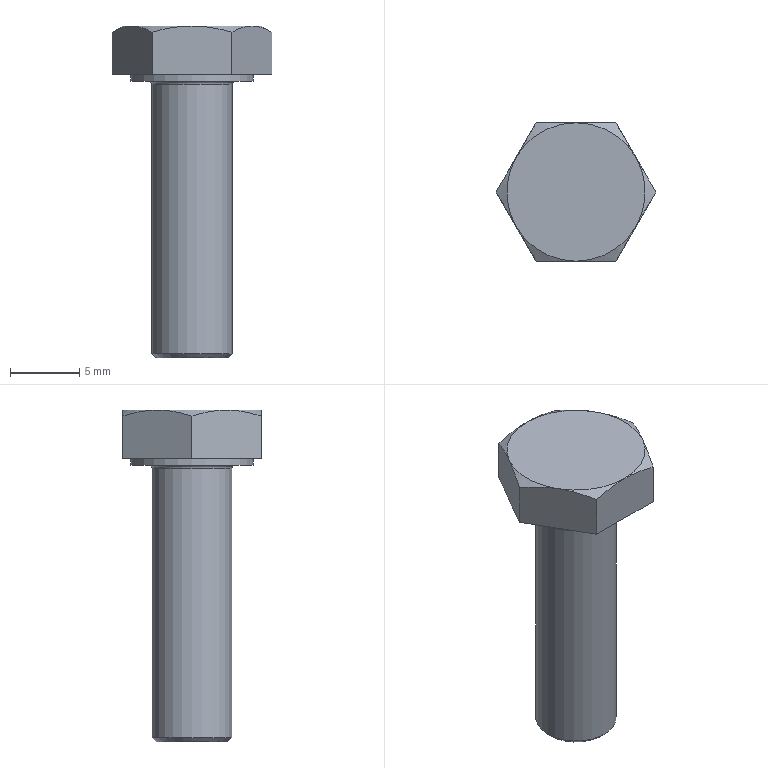Part | NX | 1 solid | 20 faces | box 11.547 x 10 x 24 mm | volume 859.994 mm3 | plane 10 | cone 7 | cylinder 2 | torus 1 | commonest cylinder face diameters 5.795 x1 8.88 x1
STEP:
#1=CARTESIAN_POINT('',(2.887,-5.,3.553));
#2=VERTEX_POINT('',#1);
#3=CARTESIAN_POINT('',(4.33,-2.5,4.));
#4=VERTEX_POINT('',#3);
#5=CARTESIAN_POINT('',(2.887,-5.,3.553));
#6=CARTESIAN_POINT('',(3.358,-4.183,3.826));
#7=CARTESIAN_POINT('',(3.837,-3.353,4.));
#8=CARTESIAN_POINT('',(4.33,-2.5,4.));
#9=B_SPLINE_CURVE_WITH_KNOTS('',3,(#5,#6,#7,#8),.UNSPECIFIED.,.F.,.F.,(4,4),(0.,1.),.UNSPECIFIED.);
#10=EDGE_CURVE('',#2,#4,#9,.T.);
#11=ORIENTED_EDGE('',*,*,#10,.F.);
#12=CARTESIAN_POINT('',(2.887,-5.,0.5));
#13=VERTEX_POINT('',#12);
#14=CARTESIAN_POINT('',(2.887,-5.,4.));
#15=DIRECTION('',(0.,0.,-1.));
#16=VECTOR('',#15,1.);
#17=LINE('',#14,#16);
#18=EDGE_CURVE('',#2,#13,#17,.T.);
#19=ORIENTED_EDGE('',*,*,#18,.T.);
#20=CARTESIAN_POINT('',(5.774,0.,0.5));
#21=VERTEX_POINT('',#20);
#22=CARTESIAN_POINT('',(2.887,-5.,0.5));
#23=DIRECTION('',(0.5,0.866,0.));
#24=VECTOR('',#23,1.);
#25=LINE('',#22,#24);
#26=EDGE_CURVE('',#13,#21,#25,.T.);
#27=ORIENTED_EDGE('',*,*,#26,.T.);
#28=CARTESIAN_POINT('',(5.774,0.,3.553));
#29=VERTEX_POINT('',#28);
#30=CARTESIAN_POINT('',(5.774,0.,4.));
#31=DIRECTION('',(0.,0.,-1.));
#32=VECTOR('',#31,1.);
#33=LINE('',#30,#32);
#34=EDGE_CURVE('',#29,#21,#33,.T.);
#35=ORIENTED_EDGE('',*,*,#34,.F.);
#36=CARTESIAN_POINT('',(4.33,-2.5,4.));
#37=CARTESIAN_POINT('',(4.823,-1.647,4.));
#38=CARTESIAN_POINT('',(5.302,-0.8168,3.826));
#39=CARTESIAN_POINT('',(5.774,0.,3.553));
#40=B_SPLINE_CURVE_WITH_KNOTS('',3,(#36,#37,#38,#39),.UNSPECIFIED.,.F.,.F.,(4,4),(0.,1.),.UNSPECIFIED.);
#41=EDGE_CURVE('',#4,#29,#40,.T.);
#42=ORIENTED_EDGE('',*,*,#41,.F.);
#43=EDGE_LOOP('',(#11,#19,#27,#35,#42));
#44=FACE_OUTER_BOUND('',#43,.T.);
#45=CARTESIAN_POINT('',(2.887,-5.,4.));
#46=DIRECTION('',(-0.866,0.5,0.));
#47=DIRECTION('',(0.5,0.866,0.));
#48=AXIS2_PLACEMENT_3D('',#45,#46,#47);
#49=PLANE('',#48);
#50=ADVANCED_FACE('',(#44),#49,.F.);
#51=CARTESIAN_POINT('',(4.33,2.5,4.));
#52=VERTEX_POINT('',#51);
#53=CARTESIAN_POINT('',(5.774,0.,3.553));
#54=CARTESIAN_POINT('',(5.302,0.8168,3.826));
#55=CARTESIAN_POINT('',(4.823,1.647,4.));
#56=CARTESIAN_POINT('',(4.33,2.5,4.));
#57=B_SPLINE_CURVE_WITH_KNOTS('',3,(#53,#54,#55,#56),.UNSPECIFIED.,.F.,.F.,(4,4),(0.,1.),.UNSPECIFIED.);
#58=EDGE_CURVE('',#29,#52,#57,.T.);
#59=ORIENTED_EDGE('',*,*,#58,.F.);
#60=ORIENTED_EDGE('',*,*,#34,.T.);
#61=CARTESIAN_POINT('',(2.887,5.,0.5));
#62=VERTEX_POINT('',#61);
#63=CARTESIAN_POINT('',(5.774,0.,0.5));
#64=DIRECTION('',(-0.5,0.866,0.));
#65=VECTOR('',#64,1.);
#66=LINE('',#63,#65);
#67=EDGE_CURVE('',#21,#62,#66,.T.);
#68=ORIENTED_EDGE('',*,*,#67,.T.);
#69=CARTESIAN_POINT('',(2.887,5.,3.553));
#70=VERTEX_POINT('',#69);
#71=CARTESIAN_POINT('',(2.887,5.,4.));
#72=DIRECTION('',(0.,0.,-1.));
#73=VECTOR('',#72,1.);
#74=LINE('',#71,#73);
#75=EDGE_CURVE('',#70,#62,#74,.T.);
#76=ORIENTED_EDGE('',*,*,#75,.F.);
#77=CARTESIAN_POINT('',(4.33,2.5,4.));
#78=CARTESIAN_POINT('',(3.837,3.353,4.));
#79=CARTESIAN_POINT('',(3.358,4.183,3.826));
#80=CARTESIAN_POINT('',(2.887,5.,3.553));
#81=B_SPLINE_CURVE_WITH_KNOTS('',3,(#77,#78,#79,#80),.UNSPECIFIED.,.F.,.F.,(4,4),(0.,1.),.UNSPECIFIED.);
#82=EDGE_CURVE('',#52,#70,#81,.T.);
#83=ORIENTED_EDGE('',*,*,#82,.F.);
#84=EDGE_LOOP('',(#59,#60,#68,#76,#83));
#85=FACE_OUTER_BOUND('',#84,.T.);
#86=CARTESIAN_POINT('',(5.774,0.,4.));
#87=DIRECTION('',(-0.866,-0.5,0.));
#88=DIRECTION('',(-0.5,0.866,0.));
#89=AXIS2_PLACEMENT_3D('',#86,#87,#88);
#90=PLANE('',#89);
#91=ADVANCED_FACE('',(#85),#90,.F.);
#92=CARTESIAN_POINT('',(0.,5.,4.));
#93=VERTEX_POINT('',#92);
#94=CARTESIAN_POINT('',(2.887,5.,3.553));
#95=CARTESIAN_POINT('',(1.944,5.,3.826));
#96=CARTESIAN_POINT('',(0.9853,5.,4.));
#97=CARTESIAN_POINT('',(0.,5.,4.));
#98=B_SPLINE_CURVE_WITH_KNOTS('',3,(#94,#95,#96,#97),.UNSPECIFIED.,.F.,.F.,(4,4),(0.,1.),.UNSPECIFIED.);
#99=EDGE_CURVE('',#70,#93,#98,.T.);
#100=ORIENTED_EDGE('',*,*,#99,.F.);
#101=ORIENTED_EDGE('',*,*,#75,.T.);
#102=CARTESIAN_POINT('',(-2.887,5.,0.5));
#103=VERTEX_POINT('',#102);
#104=CARTESIAN_POINT('',(2.887,5.,0.5));
#105=DIRECTION('',(-1.,0.,0.));
#106=VECTOR('',#105,1.);
#107=LINE('',#104,#106);
#108=EDGE_CURVE('',#62,#103,#107,.T.);
#109=ORIENTED_EDGE('',*,*,#108,.T.);
#110=CARTESIAN_POINT('',(-2.887,5.,3.553));
#111=VERTEX_POINT('',#110);
#112=CARTESIAN_POINT('',(-2.887,5.,4.));
#113=DIRECTION('',(0.,0.,-1.));
#114=VECTOR('',#113,1.);
#115=LINE('',#112,#114);
#116=EDGE_CURVE('',#111,#103,#115,.T.);
#117=ORIENTED_EDGE('',*,*,#116,.F.);
#118=CARTESIAN_POINT('',(0.,5.,4.));
#119=CARTESIAN_POINT('',(-0.9853,5.,4.));
#120=CARTESIAN_POINT('',(-1.944,5.,3.826));
#121=CARTESIAN_POINT('',(-2.887,5.,3.553));
#122=B_SPLINE_CURVE_WITH_KNOTS('',3,(#118,#119,#120,#121),.UNSPECIFIED.,.F.,.F.,(4,4),(0.,1.),.UNSPECIFIED.);
#123=EDGE_CURVE('',#93,#111,#122,.T.);
#124=ORIENTED_EDGE('',*,*,#123,.F.);
#125=EDGE_LOOP('',(#100,#101,#109,#117,#124));
#126=FACE_OUTER_BOUND('',#125,.T.);
#127=CARTESIAN_POINT('',(2.887,5.,4.));
#128=DIRECTION('',(0.,-1.,0.));
#129=DIRECTION('',(0.,0.,1.));
#130=AXIS2_PLACEMENT_3D('',#127,#128,#129);
#131=PLANE('',#130);
#132=ADVANCED_FACE('',(#126),#131,.F.);
#133=CARTESIAN_POINT('',(-4.33,2.5,4.));
#134=VERTEX_POINT('',#133);
#135=CARTESIAN_POINT('',(-2.887,5.,3.553));
#136=CARTESIAN_POINT('',(-3.358,4.183,3.826));
#137=CARTESIAN_POINT('',(-3.837,3.353,4.));
#138=CARTESIAN_POINT('',(-4.33,2.5,4.));
#139=B_SPLINE_CURVE_WITH_KNOTS('',3,(#135,#136,#137,#138),.UNSPECIFIED.,.F.,.F.,(4,4),(0.,1.),.UNSPECIFIED.);
#140=EDGE_CURVE('',#111,#134,#139,.T.);
#141=ORIENTED_EDGE('',*,*,#140,.F.);
#142=ORIENTED_EDGE('',*,*,#116,.T.);
#143=CARTESIAN_POINT('',(-5.774,0.,0.5));
#144=VERTEX_POINT('',#143);
#145=CARTESIAN_POINT('',(-2.887,5.,0.5));
#146=DIRECTION('',(-0.5,-0.866,0.));
#147=VECTOR('',#146,1.);
#148=LINE('',#145,#147);
#149=EDGE_CURVE('',#103,#144,#148,.T.);
#150=ORIENTED_EDGE('',*,*,#149,.T.);
#151=CARTESIAN_POINT('',(-5.774,0.,3.553));
#152=VERTEX_POINT('',#151);
#153=CARTESIAN_POINT('',(-5.774,0.,4.));
#154=DIRECTION('',(0.,0.,-1.));
#155=VECTOR('',#154,1.);
#156=LINE('',#153,#155);
#157=EDGE_CURVE('',#152,#144,#156,.T.);
#158=ORIENTED_EDGE('',*,*,#157,.F.);
#159=CARTESIAN_POINT('',(-4.33,2.5,4.));
#160=CARTESIAN_POINT('',(-4.823,1.647,4.));
#161=CARTESIAN_POINT('',(-5.302,0.8168,3.826));
#162=CARTESIAN_POINT('',(-5.774,0.,3.553));
#163=B_SPLINE_CURVE_WITH_KNOTS('',3,(#159,#160,#161,#162),.UNSPECIFIED.,.F.,.F.,(4,4),(0.,1.),.UNSPECIFIED.);
#164=EDGE_CURVE('',#134,#152,#163,.T.);
#165=ORIENTED_EDGE('',*,*,#164,.F.);
#166=EDGE_LOOP('',(#141,#142,#150,#158,#165));
#167=FACE_OUTER_BOUND('',#166,.T.);
#168=CARTESIAN_POINT('',(-2.887,5.,4.));
#169=DIRECTION('',(0.866,-0.5,0.));
#170=DIRECTION('',(-0.5,-0.866,0.));
#171=AXIS2_PLACEMENT_3D('',#168,#169,#170);
#172=PLANE('',#171);
#173=ADVANCED_FACE('',(#167),#172,.F.);
#174=CARTESIAN_POINT('',(-4.33,-2.5,4.));
#175=VERTEX_POINT('',#174);
#176=CARTESIAN_POINT('',(-5.774,0.,3.553));
#177=CARTESIAN_POINT('',(-5.302,-0.8168,3.826));
#178=CARTESIAN_POINT('',(-4.823,-1.647,4.));
#179=CARTESIAN_POINT('',(-4.33,-2.5,4.));
#180=B_SPLINE_CURVE_WITH_KNOTS('',3,(#176,#177,#178,#179),.UNSPECIFIED.,.F.,.F.,(4,4),(0.,1.),.UNSPECIFIED.);
#181=EDGE_CURVE('',#152,#175,#180,.T.);
#182=ORIENTED_EDGE('',*,*,#181,.F.);
#183=ORIENTED_EDGE('',*,*,#157,.T.);
#184=CARTESIAN_POINT('',(-2.887,-5.,0.5));
#185=VERTEX_POINT('',#184);
#186=CARTESIAN_POINT('',(-5.774,0.,0.5));
#187=DIRECTION('',(0.5,-0.866,0.));
#188=VECTOR('',#187,1.);
#189=LINE('',#186,#188);
#190=EDGE_CURVE('',#144,#185,#189,.T.);
#191=ORIENTED_EDGE('',*,*,#190,.T.);
#192=CARTESIAN_POINT('',(-2.887,-5.,3.553));
#193=VERTEX_POINT('',#192);
#194=CARTESIAN_POINT('',(-2.887,-5.,4.));
#195=DIRECTION('',(0.,0.,-1.));
#196=VECTOR('',#195,1.);
#197=LINE('',#194,#196);
#198=EDGE_CURVE('',#193,#185,#197,.T.);
#199=ORIENTED_EDGE('',*,*,#198,.F.);
#200=CARTESIAN_POINT('',(-4.33,-2.5,4.));
#201=CARTESIAN_POINT('',(-3.837,-3.353,4.));
#202=CARTESIAN_POINT('',(-3.358,-4.183,3.826));
#203=CARTESIAN_POINT('',(-2.887,-5.,3.553));
#204=B_SPLINE_CURVE_WITH_KNOTS('',3,(#200,#201,#202,#203),.UNSPECIFIED.,.F.,.F.,(4,4),(0.,1.),.UNSPECIFIED.);
#205=EDGE_CURVE('',#175,#193,#204,.T.);
#206=ORIENTED_EDGE('',*,*,#205,.F.);
#207=EDGE_LOOP('',(#182,#183,#191,#199,#206));
#208=FACE_OUTER_BOUND('',#207,.T.);
#209=CARTESIAN_POINT('',(-5.774,0.,4.));
#210=DIRECTION('',(0.866,0.5,0.));
#211=DIRECTION('',(0.5,-0.866,0.));
#212=AXIS2_PLACEMENT_3D('',#209,#210,#211);
#213=PLANE('',#212);
#214=ADVANCED_FACE('',(#208),#213,.F.);
#215=CARTESIAN_POINT('',(0.,-5.,4.));
#216=VERTEX_POINT('',#215);
#217=CARTESIAN_POINT('',(-2.887,-5.,3.553));
#218=CARTESIAN_POINT('',(-1.944,-5.,3.826));
#219=CARTESIAN_POINT('',(-0.9853,-5.,4.));
#220=CARTESIAN_POINT('',(0.,-5.,4.));
#221=B_SPLINE_CURVE_WITH_KNOTS('',3,(#217,#218,#219,#220),.UNSPECIFIED.,.F.,.F.,(4,4),(0.,1.),.UNSPECIFIED.);
#222=EDGE_CURVE('',#193,#216,#221,.T.);
#223=ORIENTED_EDGE('',*,*,#222,.F.);
#224=ORIENTED_EDGE('',*,*,#198,.T.);
#225=CARTESIAN_POINT('',(-2.887,-5.,0.5));
#226=DIRECTION('',(1.,0.,0.));
#227=VECTOR('',#226,1.);
#228=LINE('',#225,#227);
#229=EDGE_CURVE('',#185,#13,#228,.T.);
#230=ORIENTED_EDGE('',*,*,#229,.T.);
#231=ORIENTED_EDGE('',*,*,#18,.F.);
#232=CARTESIAN_POINT('',(0.,-5.,4.));
#233=CARTESIAN_POINT('',(0.9853,-5.,4.));
#234=CARTESIAN_POINT('',(1.944,-5.,3.826));
#235=CARTESIAN_POINT('',(2.887,-5.,3.553));
#236=B_SPLINE_CURVE_WITH_KNOTS('',3,(#232,#233,#234,#235),.UNSPECIFIED.,.F.,.F.,(4,4),(0.,1.),.UNSPECIFIED.);
#237=EDGE_CURVE('',#216,#2,#236,.T.);
#238=ORIENTED_EDGE('',*,*,#237,.F.);
#239=EDGE_LOOP('',(#223,#224,#230,#231,#238));
#240=FACE_OUTER_BOUND('',#239,.T.);
#241=CARTESIAN_POINT('',(-2.887,-5.,4.));
#242=DIRECTION('',(0.,1.,0.));
#243=DIRECTION('',(1.,0.,0.));
#244=AXIS2_PLACEMENT_3D('',#241,#242,#243);
#245=PLANE('',#244);
#246=ADVANCED_FACE('',(#240),#245,.F.);
#247=CARTESIAN_POINT('',(4.44,0.,0.5));
#248=VERTEX_POINT('',#247);
#249=CARTESIAN_POINT('',(0.,0.,0.5));
#250=DIRECTION('',(0.,0.,1.));
#251=DIRECTION('',(1.,0.,0.));
#252=AXIS2_PLACEMENT_3D('',#249,#250,#251);
#253=CIRCLE('',#252,4.44);
#254=EDGE_CURVE('',#248,#248,#253,.T.);
#255=ORIENTED_EDGE('',*,*,#254,.T.);
#256=EDGE_LOOP('',(#255));
#257=FACE_BOUND('',#256,.T.);
#258=ORIENTED_EDGE('',*,*,#26,.F.);
#259=ORIENTED_EDGE('',*,*,#229,.F.);
#260=ORIENTED_EDGE('',*,*,#190,.F.);
#261=ORIENTED_EDGE('',*,*,#149,.F.);
#262=ORIENTED_EDGE('',*,*,#108,.F.);
#263=ORIENTED_EDGE('',*,*,#67,.F.);
#264=EDGE_LOOP('',(#258,#259,#260,#261,#262,#263));
#265=FACE_BOUND('',#264,.T.);
#266=CARTESIAN_POINT('',(8.66,5.,0.5));
#267=DIRECTION('',(0.,0.,1.));
#268=DIRECTION('',(-1.,0.,0.));
#269=AXIS2_PLACEMENT_3D('',#266,#267,#268);
#270=PLANE('',#269);
#271=ADVANCED_FACE('',(#257,#265),#270,.F.);
#272=ORIENTED_EDGE('',*,*,#10,.T.);
#273=CARTESIAN_POINT('',(0.,0.,4.));
#274=DIRECTION('',(0.,0.,-1.));
#275=DIRECTION('',(-1.,0.,0.));
#276=AXIS2_PLACEMENT_3D('',#273,#274,#275);
#277=CIRCLE('',#276,5.);
#278=EDGE_CURVE('',#4,#216,#277,.T.);
#279=ORIENTED_EDGE('',*,*,#278,.T.);
#280=ORIENTED_EDGE('',*,*,#237,.T.);
#281=EDGE_LOOP('',(#272,#279,#280));
#282=FACE_OUTER_BOUND('',#281,.T.);
#283=CARTESIAN_POINT('',(0.,0.,3.553));
#284=DIRECTION('',(0.,0.,-1.));
#285=DIRECTION('',(1.,0.,0.));
#286=AXIS2_PLACEMENT_3D('',#283,#284,#285);
#287=CONICAL_SURFACE('',#286,5.774,60.);
#288=ADVANCED_FACE('',(#282),#287,.T.);
#289=ORIENTED_EDGE('',*,*,#205,.T.);
#290=ORIENTED_EDGE('',*,*,#222,.T.);
#291=CARTESIAN_POINT('',(0.,0.,4.));
#292=DIRECTION('',(0.,0.,-1.));
#293=DIRECTION('',(-1.,0.,0.));
#294=AXIS2_PLACEMENT_3D('',#291,#292,#293);
#295=CIRCLE('',#294,5.);
#296=EDGE_CURVE('',#216,#175,#295,.T.);
#297=ORIENTED_EDGE('',*,*,#296,.T.);
#298=EDGE_LOOP('',(#289,#290,#297));
#299=FACE_OUTER_BOUND('',#298,.T.);
#300=CARTESIAN_POINT('',(0.,0.,3.553));
#301=DIRECTION('',(0.,0.,-1.));
#302=DIRECTION('',(1.,0.,0.));
#303=AXIS2_PLACEMENT_3D('',#300,#301,#302);
#304=CONICAL_SURFACE('',#303,5.774,60.);
#305=ADVANCED_FACE('',(#299),#304,.T.);
#306=ORIENTED_EDGE('',*,*,#164,.T.);
#307=ORIENTED_EDGE('',*,*,#181,.T.);
#308=CARTESIAN_POINT('',(0.,0.,4.));
#309=DIRECTION('',(0.,0.,-1.));
#310=DIRECTION('',(-1.,0.,0.));
#311=AXIS2_PLACEMENT_3D('',#308,#309,#310);
#312=CIRCLE('',#311,5.);
#313=EDGE_CURVE('',#175,#134,#312,.T.);
#314=ORIENTED_EDGE('',*,*,#313,.T.);
#315=EDGE_LOOP('',(#306,#307,#314));
#316=FACE_OUTER_BOUND('',#315,.T.);
#317=CARTESIAN_POINT('',(0.,0.,3.553));
#318=DIRECTION('',(0.,0.,-1.));
#319=DIRECTION('',(1.,0.,0.));
#320=AXIS2_PLACEMENT_3D('',#317,#318,#319);
#321=CONICAL_SURFACE('',#320,5.774,60.);
#322=ADVANCED_FACE('',(#316),#321,.T.);
#323=ORIENTED_EDGE('',*,*,#123,.T.);
#324=ORIENTED_EDGE('',*,*,#140,.T.);
#325=CARTESIAN_POINT('',(0.,0.,4.));
#326=DIRECTION('',(0.,0.,-1.));
#327=DIRECTION('',(-1.,0.,0.));
#328=AXIS2_PLACEMENT_3D('',#325,#326,#327);
#329=CIRCLE('',#328,5.);
#330=EDGE_CURVE('',#134,#93,#329,.T.);
#331=ORIENTED_EDGE('',*,*,#330,.T.);
#332=EDGE_LOOP('',(#323,#324,#331));
#333=FACE_OUTER_BOUND('',#332,.T.);
#334=CARTESIAN_POINT('',(0.,0.,3.553));
#335=DIRECTION('',(0.,0.,-1.));
#336=DIRECTION('',(1.,0.,0.));
#337=AXIS2_PLACEMENT_3D('',#334,#335,#336);
#338=CONICAL_SURFACE('',#337,5.774,60.);
#339=ADVANCED_FACE('',(#333),#338,.T.);
#340=ORIENTED_EDGE('',*,*,#82,.T.);
#341=ORIENTED_EDGE('',*,*,#99,.T.);
#342=CARTESIAN_POINT('',(0.,0.,4.));
#343=DIRECTION('',(0.,0.,-1.));
#344=DIRECTION('',(-1.,0.,0.));
#345=AXIS2_PLACEMENT_3D('',#342,#343,#344);
#346=CIRCLE('',#345,5.);
#347=EDGE_CURVE('',#93,#52,#346,.T.);
#348=ORIENTED_EDGE('',*,*,#347,.T.);
#349=EDGE_LOOP('',(#340,#341,#348));
#350=FACE_OUTER_BOUND('',#349,.T.);
#351=CARTESIAN_POINT('',(0.,0.,3.553));
#352=DIRECTION('',(0.,0.,-1.));
#353=DIRECTION('',(1.,0.,0.));
#354=AXIS2_PLACEMENT_3D('',#351,#352,#353);
#355=CONICAL_SURFACE('',#354,5.774,60.);
#356=ADVANCED_FACE('',(#350),#355,.T.);
#357=ORIENTED_EDGE('',*,*,#41,.T.);
#358=ORIENTED_EDGE('',*,*,#58,.T.);
#359=CARTESIAN_POINT('',(0.,0.,4.));
#360=DIRECTION('',(0.,0.,-1.));
#361=DIRECTION('',(-1.,0.,0.));
#362=AXIS2_PLACEMENT_3D('',#359,#360,#361);
#363=CIRCLE('',#362,5.);
#364=EDGE_CURVE('',#52,#4,#363,.T.);
#365=ORIENTED_EDGE('',*,*,#364,.T.);
#366=EDGE_LOOP('',(#357,#358,#365));
#367=FACE_OUTER_BOUND('',#366,.T.);
#368=CARTESIAN_POINT('',(0.,0.,3.553));
#369=DIRECTION('',(0.,0.,-1.));
#370=DIRECTION('',(1.,0.,0.));
#371=AXIS2_PLACEMENT_3D('',#368,#369,#370);
#372=CONICAL_SURFACE('',#371,5.774,60.);
#373=ADVANCED_FACE('',(#367),#372,.T.);
#374=ORIENTED_EDGE('',*,*,#330,.F.);
#375=ORIENTED_EDGE('',*,*,#313,.F.);
#376=ORIENTED_EDGE('',*,*,#296,.F.);
#377=ORIENTED_EDGE('',*,*,#278,.F.);
#378=ORIENTED_EDGE('',*,*,#364,.F.);
#379=ORIENTED_EDGE('',*,*,#347,.F.);
#380=EDGE_LOOP('',(#374,#375,#376,#377,#378,#379));
#381=FACE_OUTER_BOUND('',#380,.T.);
#382=CARTESIAN_POINT('',(8.66,5.,4.));
#383=DIRECTION('',(0.,0.,1.));
#384=DIRECTION('',(-1.,0.,0.));
#385=AXIS2_PLACEMENT_3D('',#382,#383,#384);
#386=PLANE('',#385);
#387=ADVANCED_FACE('',(#381),#386,.T.);
#388=ORIENTED_EDGE('',*,*,#254,.F.);
#389=EDGE_LOOP('',(#388));
#390=FACE_BOUND('',#389,.T.);
#391=CARTESIAN_POINT('',(4.44,0.,0.));
#392=VERTEX_POINT('',#391);
#393=CARTESIAN_POINT('',(0.,0.,0.));
#394=DIRECTION('',(0.,0.,1.));
#395=DIRECTION('',(1.,0.,0.));
#396=AXIS2_PLACEMENT_3D('',#393,#394,#395);
#397=CIRCLE('',#396,4.44);
#398=EDGE_CURVE('',#392,#392,#397,.T.);
#399=ORIENTED_EDGE('',*,*,#398,.T.);
#400=EDGE_LOOP('',(#399));
#401=FACE_BOUND('',#400,.T.);
#402=CARTESIAN_POINT('',(0.,0.,0.5));
#403=DIRECTION('',(0.,0.,-1.));
#404=DIRECTION('',(1.,0.,0.));
#405=AXIS2_PLACEMENT_3D('',#402,#403,#404);
#406=CYLINDRICAL_SURFACE('',#405,4.44);
#407=ADVANCED_FACE('',(#390,#401),#406,.T.);
#408=CARTESIAN_POINT('',(3.147,0.,0.));
#409=VERTEX_POINT('',#408);
#410=CARTESIAN_POINT('',(0.,0.,0.));
#411=DIRECTION('',(0.,0.,1.));
#412=DIRECTION('',(1.,0.,0.));
#413=AXIS2_PLACEMENT_3D('',#410,#411,#412);
#414=CIRCLE('',#413,3.147);
#415=EDGE_CURVE('',#409,#409,#414,.T.);
#416=ORIENTED_EDGE('',*,*,#415,.T.);
#417=EDGE_LOOP('',(#416));
#418=FACE_BOUND('',#417,.T.);
#419=ORIENTED_EDGE('',*,*,#398,.F.);
#420=EDGE_LOOP('',(#419));
#421=FACE_BOUND('',#420,.T.);
#422=CARTESIAN_POINT('',(0.,0.,0.));
#423=DIRECTION('',(0.,0.,1.));
#424=DIRECTION('',(-1.,0.,0.));
#425=AXIS2_PLACEMENT_3D('',#422,#423,#424);
#426=PLANE('',#425);
#427=ADVANCED_FACE('',(#418,#421),#426,.F.);
#428=CARTESIAN_POINT('',(2.897,0.,-0.25));
#429=VERTEX_POINT('',#428);
#430=CARTESIAN_POINT('',(0.,0.,-0.25));
#431=DIRECTION('',(0.,0.,-1.));
#432=DIRECTION('',(1.,0.,0.));
#433=AXIS2_PLACEMENT_3D('',#430,#431,#432);
#434=CIRCLE('',#433,2.897);
#435=EDGE_CURVE('',#429,#429,#434,.T.);
#436=ORIENTED_EDGE('',*,*,#435,.T.);
#437=EDGE_LOOP('',(#436));
#438=FACE_BOUND('',#437,.T.);
#439=CARTESIAN_POINT('',(2.897,0.,-19.71));
#440=VERTEX_POINT('',#439);
#441=CARTESIAN_POINT('',(0.,0.,-19.71));
#442=DIRECTION('',(0.,0.,1.));
#443=DIRECTION('',(1.,0.,0.));
#444=AXIS2_PLACEMENT_3D('',#441,#442,#443);
#445=CIRCLE('',#444,2.897);
#446=EDGE_CURVE('',#440,#440,#445,.T.);
#447=ORIENTED_EDGE('',*,*,#446,.T.);
#448=EDGE_LOOP('',(#447));
#449=FACE_BOUND('',#448,.T.);
#450=CARTESIAN_POINT('',(0.,0.,-20.));
#451=DIRECTION('',(0.,0.,1.));
#452=DIRECTION('',(-1.,0.,0.));
#453=AXIS2_PLACEMENT_3D('',#450,#451,#452);
#454=CYLINDRICAL_SURFACE('',#453,2.897);
#455=ADVANCED_FACE('',(#438,#449),#454,.T.);
#456=CARTESIAN_POINT('',(2.608,0.,-20.));
#457=VERTEX_POINT('',#456);
#458=CARTESIAN_POINT('',(0.,0.,-20.));
#459=DIRECTION('',(0.,0.,-1.));
#460=DIRECTION('',(1.,0.,0.));
#461=AXIS2_PLACEMENT_3D('',#458,#459,#460);
#462=CIRCLE('',#461,2.608);
#463=EDGE_CURVE('',#457,#457,#462,.T.);
#464=ORIENTED_EDGE('',*,*,#463,.T.);
#465=EDGE_LOOP('',(#464));
#466=FACE_OUTER_BOUND('',#465,.T.);
#467=CARTESIAN_POINT('',(0.,0.,-20.));
#468=DIRECTION('',(0.,0.,1.));
#469=DIRECTION('',(-1.,0.,0.));
#470=AXIS2_PLACEMENT_3D('',#467,#468,#469);
#471=PLANE('',#470);
#472=ADVANCED_FACE('',(#466),#471,.F.);
#473=ORIENTED_EDGE('',*,*,#463,.F.);
#474=EDGE_LOOP('',(#473));
#475=FACE_BOUND('',#474,.T.);
#476=ORIENTED_EDGE('',*,*,#446,.F.);
#477=EDGE_LOOP('',(#476));
#478=FACE_BOUND('',#477,.T.);
#479=CARTESIAN_POINT('',(0.,0.,-19.71));
#480=DIRECTION('',(0.,0.,1.));
#481=DIRECTION('',(-1.,0.,0.));
#482=AXIS2_PLACEMENT_3D('',#479,#480,#481);
#483=CONICAL_SURFACE('',#482,2.897,45.);
#484=ADVANCED_FACE('',(#475,#478),#483,.T.);
#485=ORIENTED_EDGE('',*,*,#435,.F.);
#486=EDGE_LOOP('',(#485));
#487=FACE_BOUND('',#486,.T.);
#488=ORIENTED_EDGE('',*,*,#415,.F.);
#489=EDGE_LOOP('',(#488));
#490=FACE_BOUND('',#489,.T.);
#491=CARTESIAN_POINT('',(0.,0.,-0.25));
#492=DIRECTION('',(0.,0.,1.));
#493=DIRECTION('',(-1.,0.,0.));
#494=AXIS2_PLACEMENT_3D('',#491,#492,#493);
#495=TOROIDAL_SURFACE('',#494,3.147,0.25);
#496=ADVANCED_FACE('',(#487,#490),#495,.F.);
#497=CLOSED_SHELL('',(#50,#91,#132,#173,#214,#246,#271,#288,#305,#322,#339,#356,#373,#387,#407,#427,#455,#472,#484,#496));
#498=MANIFOLD_SOLID_BREP('',#497);
#499=(LENGTH_UNIT()NAMED_UNIT(*)SI_UNIT(.MILLI.,.METRE.));
#500=UNCERTAINTY_MEASURE_WITH_UNIT(LENGTH_MEASURE(0.0508),#499,'','');
#501=(NAMED_UNIT(*)PLANE_ANGLE_UNIT()SI_UNIT($,.RADIAN.));
#502=PLANE_ANGLE_MEASURE_WITH_UNIT(PLANE_ANGLE_MEASURE(0.01745),#501);
#503=DIMENSIONAL_EXPONENTS(0.,0.,0.,0.,0.,0.,0.);
#504=(CONVERSION_BASED_UNIT('DEGREE',#502)NAMED_UNIT(#503)PLANE_ANGLE_UNIT());
#505=(NAMED_UNIT(*)SI_UNIT($,.STERADIAN.)SOLID_ANGLE_UNIT());
#506=(GEOMETRIC_REPRESENTATION_CONTEXT(3)GLOBAL_UNCERTAINTY_ASSIGNED_CONTEXT((#500))GLOBAL_UNIT_ASSIGNED_CONTEXT((#499,#504,#505))REPRESENTATION_CONTEXT('',''));
#507=ADVANCED_BREP_SHAPE_REPRESENTATION('',(#498),#506);